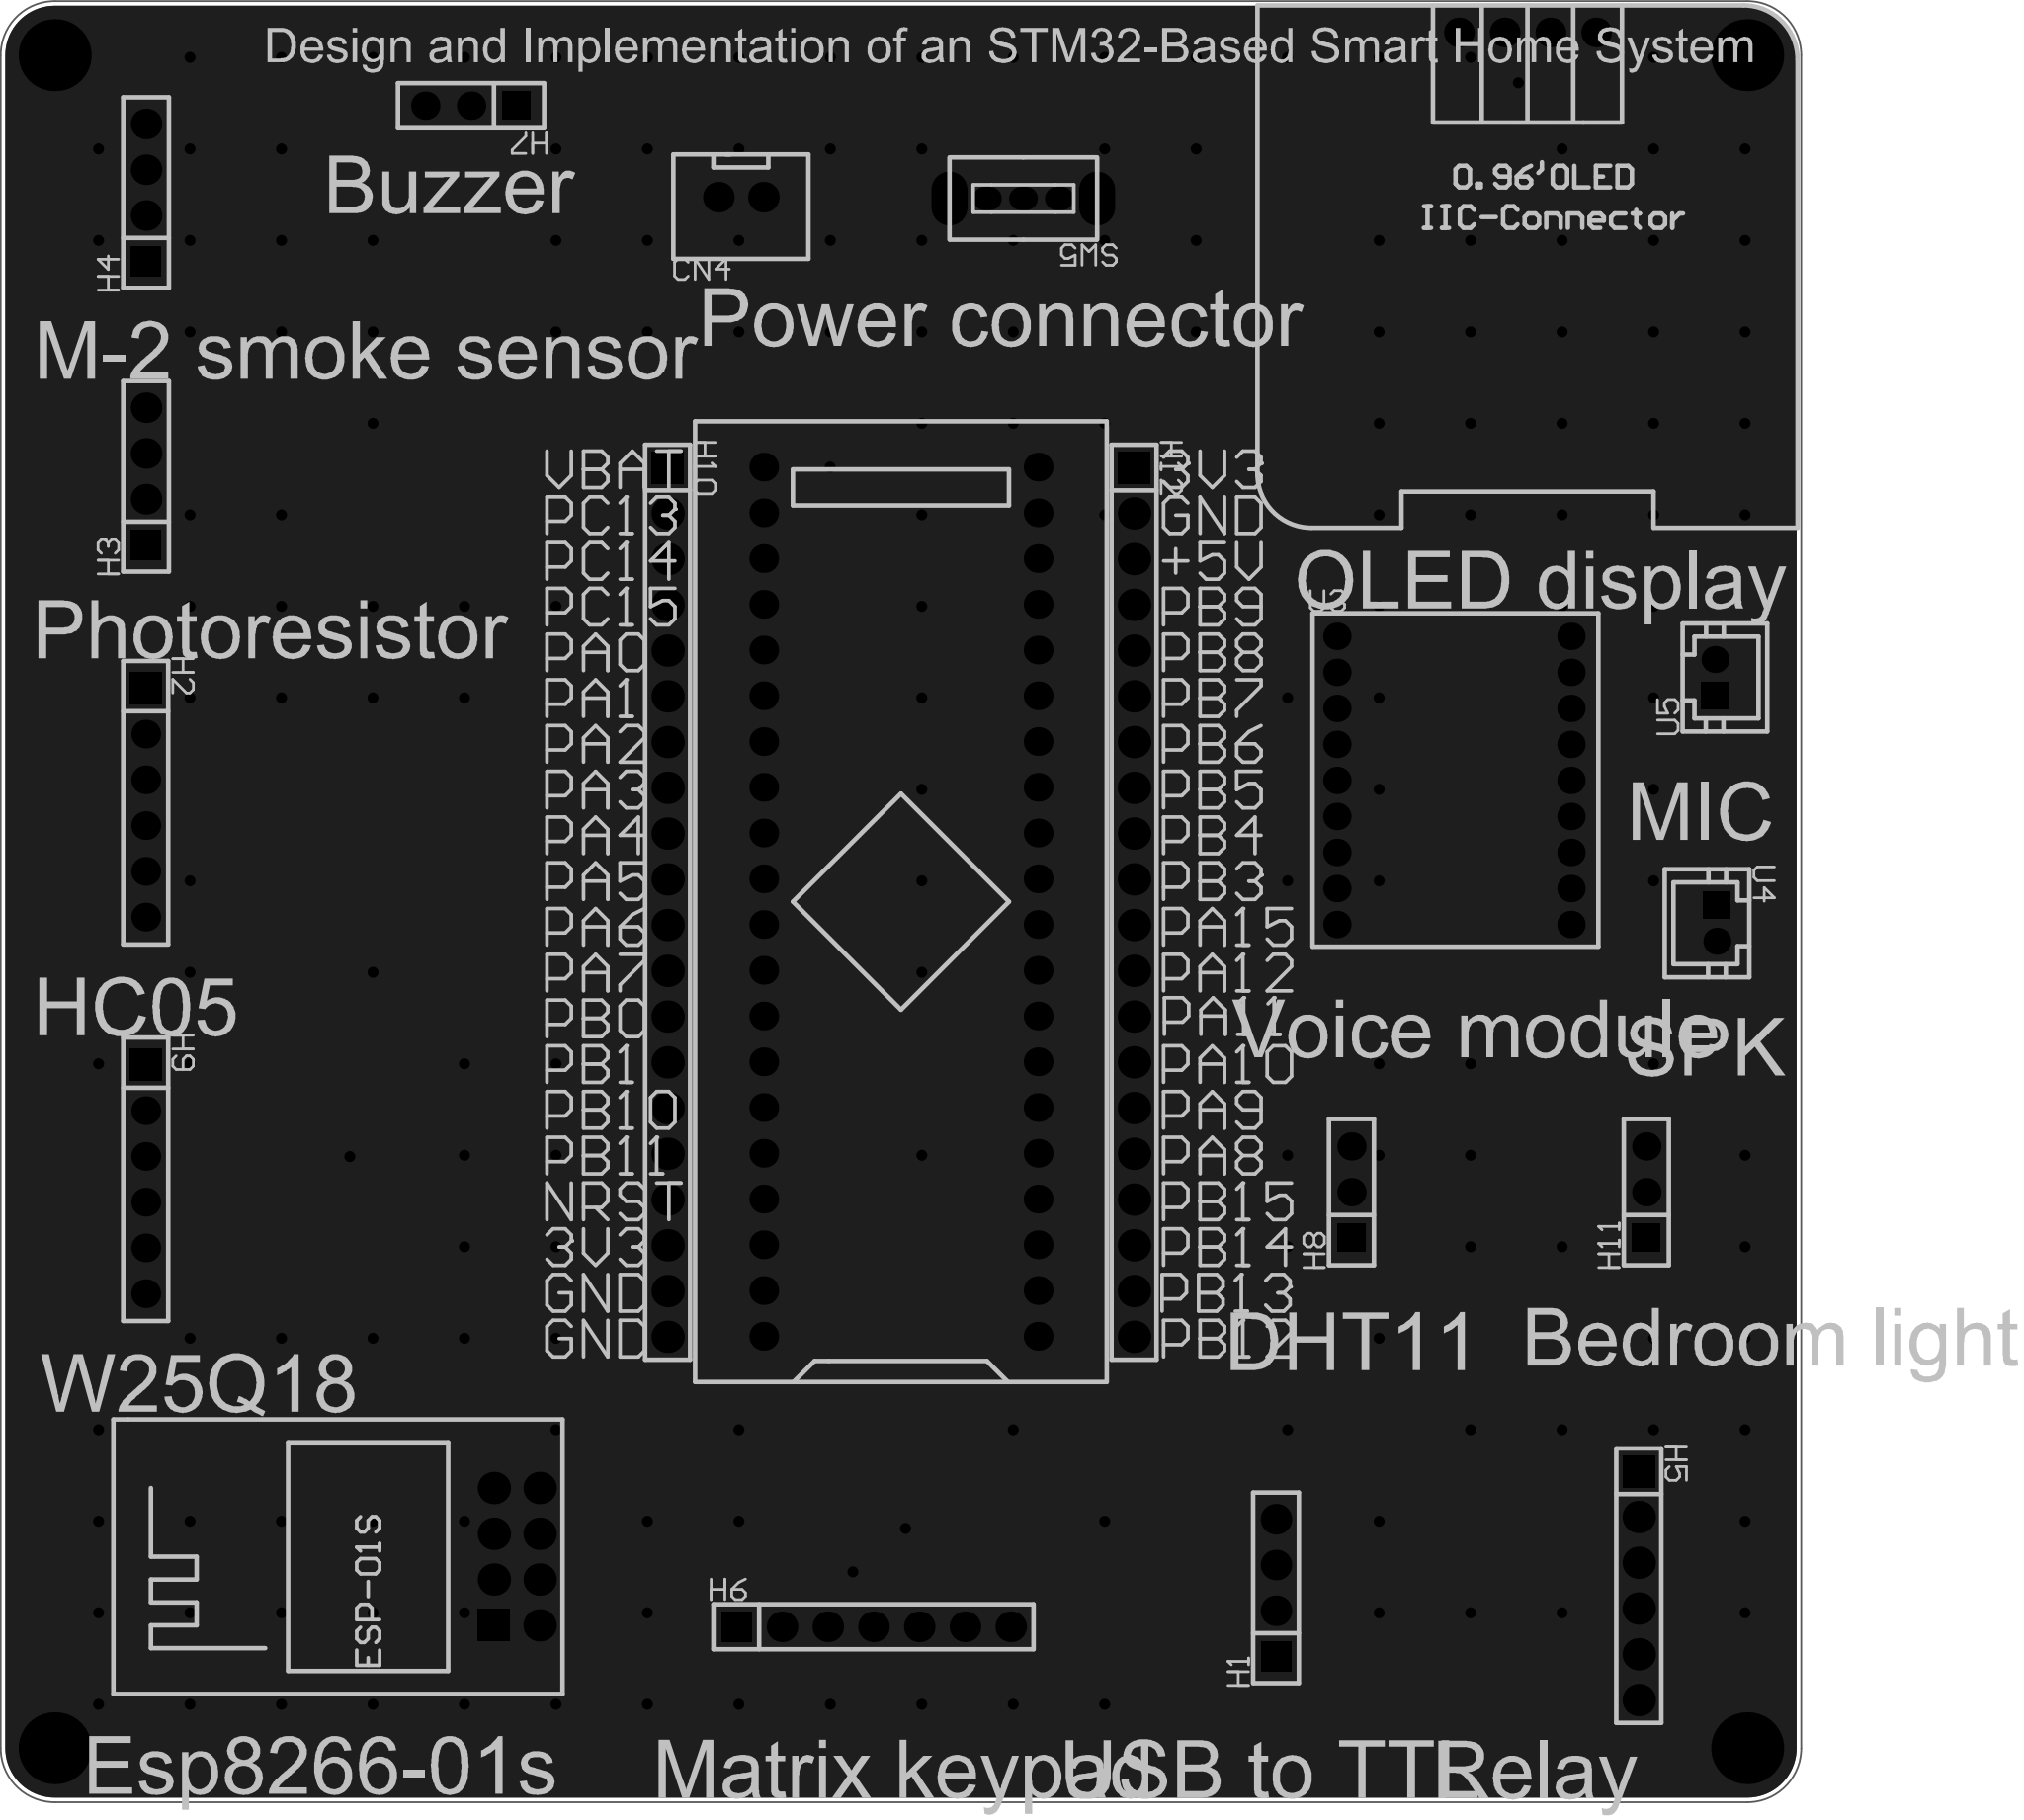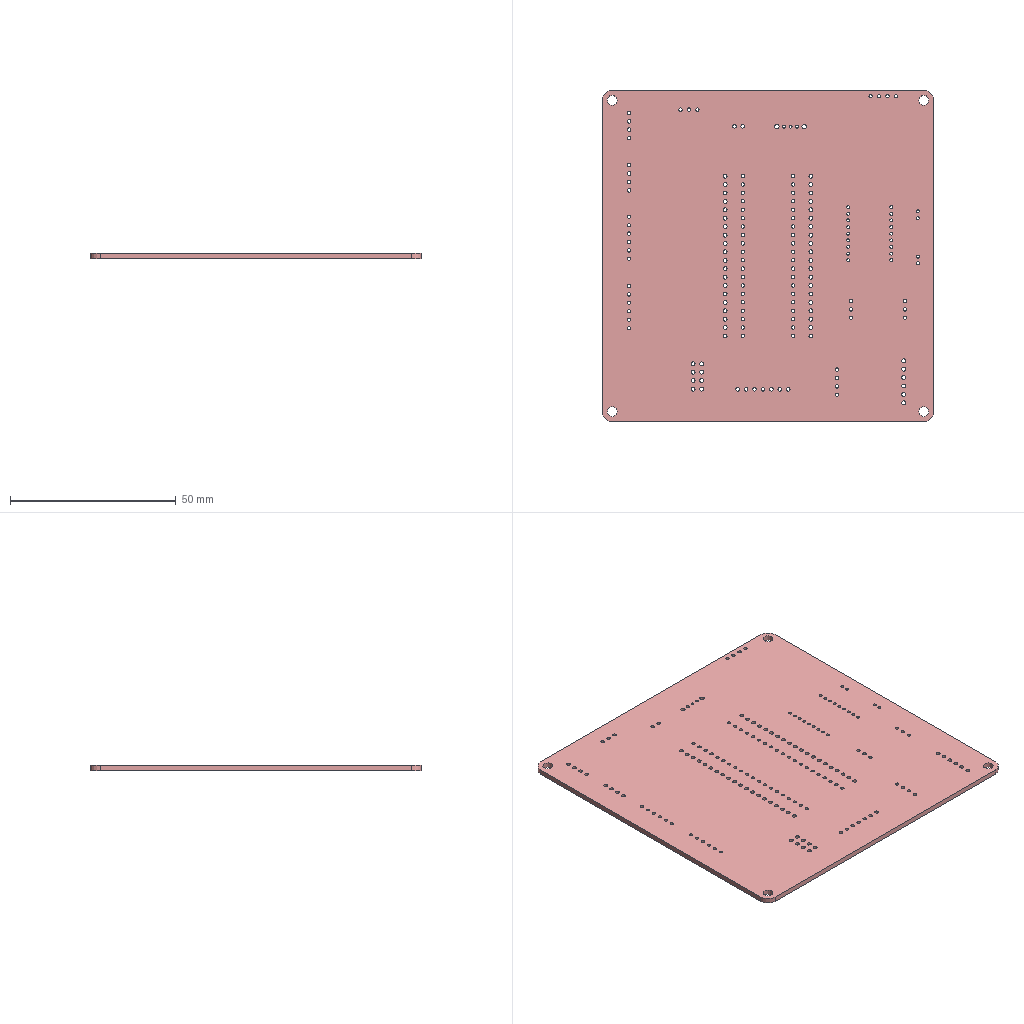Circuit board layout | Altium Designer | box 100 x 100 x 1.6 mm
Layer stack:
# Altium Designer layer stack of  (unit mm; dielectric type: 0 none, 1 core, 2 prepreg, 3 surface material)
index,name,kind,layer,copper_thickness_mm,dielectric_type,dielectric_thickness_mm,dielectric_material,dielectric_constant
0,Top Paste Mask Layer,other,,,,,,
1,Top Silkscreen Layer,other,,,,,,
2,Top Solder Mask Layer,dielectric,,,3,0.01,,3.3
3,Top Layer,copper,Top Layer,0.035,,,,
4,Dielectric1,dielectric,,,3,1.51,FR4,4.5
5,Bottom Layer,copper,Bottom Layer,0.035,,,,
6,Bottom Solder Mask Layer,dielectric,,,3,0.01,,3.3
7,Bottom Silkscreen Layer,other,,,,,,
8,Bottom Paste Mask Layer,other,,,,,,
# drill layer pairs: low layer,high layer
drill_pair,Top Layer,Bottom Layer
Part placement:
Designator,Comment,Layer,Footprint,Center-X(mm),Center-Y(mm),Rotation
U1,STM32F103C8T6-Card,TopLayer,CONN-TH_L53.3-W22.9_STM32F103C8T6-CARD,141.351,130.937,90
U2,ESP-01S,TopLayer,WIFIM-TH_ESP-01S,120.015,94.57,90
OLED1,,TopLayer,0.96OLED_4P,176.149,179.197,0
H11,,TopLayer,HDR-TH_3P-P2.54-V-F,182.746,114.808,90
CN4,XH2.54*2P_THT,TopLayer,CONN-TH_2P-P2.50-XH2.54-2P,132.461,170.053,0
U3,CON2.0MM-PAD-18,TopLayer,CONN-TH_18P-P2.00_C9900078766,172.062,137.668,90
SW5,,TopLayer,拨动开关,148.148,169.978,180
H1,,TopLayer,HDR-TH_4P-P2.54-V-F,162.179,92.837,90
H2,,TopLayer,HDR-TH_6P-P2.54-V-F,99.406,136.431,270
H3,,TopLayer,HDR-TH_4P-P2.54-V-F,99.426,154.553,90
H4,,TopLayer,HDR-TH_4P-P2.54-V-F,99.426,170.307,90
H5,,TopLayer,HDR-TH_6P-P2.54-V-M-1,182.328,92.962,270
H6,,TopLayer,HDR-TH_7P-P2.54-V-M,139.827,90.678,0
H7,,TopLayer,HDR-TH_3P-P2.54-V-F,117.475,175.133,180
H8,,TopLayer,HDR-TH_3P-P2.54-V-F,166.37,114.808,90
H9,,TopLayer,HDR-TH_6P-P2.54-V-F,99.406,115.524,270
H10,,TopLayer,HDR-TH_20P-P2.54-V-M-1,128.394,130.907,270
H12,,TopLayer,HDR-TH_20P-P2.54-V-M-1,154.294,130.907,270
U4,PH2.0-2P,TopLayer,CONN-TH_2P-P2.00_BOSSIE_BX-PH2.0-2PZZ,186.666,129.738,270
U5,PH2.0-2P,TopLayer,CONN-TH_2P-P2.00_BOSSIE_BX-PH2.0-2PZZ,186.563,143.383,90
Pad and via stacks:
# Altium Designer via and pad stacks of  (unit mm). Each distinct definition once, with the count of objects using it.
# via: kind,start_layer,end_layer,hole_mm,diameter_mm,mode(0 simple;1 top-mid-bottom;2 full stack),diameter_per_layer,count,example_net
# pad: kind,layer,hole_mm,hole_type(0 round;1 square;2 slot),plating,top_size,top_shape(1 round;2 rect;3 octagon;9 rounded rect),mid_size,bottom_size,mode,footprint,size_per_layer,count,example
pad,Multi-Layer,3,0,plated,4x4,1,4x4,4x4,0,,,4,1
pad,Multi-Layer,1,0,plated,1.6x1.6,1,1.6x1.6,1.6x1.6,0,CONN-TH_L53.3-W22.9_STM32F103C8T6-CARD,,40,U1.1
pad,Multi-Layer,1.2,0,plated,1.8x1.8,2,1.8x1.8,1.8x1.8,0,WIFIM-TH_ESP-01S,,1,U2.1
pad,Multi-Layer,1.2,0,plated,1.8x1.8,1,1.8x1.8,1.8x1.8,0,WIFIM-TH_ESP-01S,,7,U2.2
pad,Multi-Layer,1,0,plated,1.65x1.65,1,1.65x1.65,1.65x1.65,0,0.96OLED_4P,,4,OLED1.4
pad,Multi-Layer,1.02,0,plated,1.575x1.575,1,1.575x1.575,1.575x1.575,0,HDR-TH_3P-P2.54-V-F,,6,H11.3
pad,Multi-Layer,1.02,0,plated,1.575x1.575,2,1.575x1.575,1.575x1.575,0,HDR-TH_3P-P2.54-V-F,,3,H11.1
pad,Multi-Layer,1.05,0,plated,1.7x1.7,1,1.7x1.7,1.7x1.7,0,CONN-TH_2P-P2.50-XH2.54-2P,,2,CN4.2
pad,Multi-Layer,0.9,0,plated,1.524x1.524,1,1.524x1.524,1.524x1.524,0,CONN-TH_18P-P2.00_C9900078766,,18,U3.1
pad,Multi-Layer,0.8992,0,plated,1.6x1.3,1,1.6x1.3,1.6x1.3,0,\u00B2\u00A6\u00B6\u00AF\u00BF\u00AA\u00B9\u00D8,,3,SW5.1
pad,Multi-Layer,1.3,0,plated,3x1.999,1,3x1.999,3x1.999,0,\u00B2\u00A6\u00B6\u00AF\u00BF\u00AA\u00B9\u00D8,,2,SW5.4
pad,Multi-Layer,1.1,0,plated,1.7x1.7,2,1.7x1.7,1.7x1.7,0,HDR-TH_4P-P2.54-V-F,,3,H1.1
pad,Multi-Layer,1.1,0,plated,1.7x1.7,1,1.7x1.7,1.7x1.7,0,HDR-TH_4P-P2.54-V-F,,9,H1.2
pad,Multi-Layer,1.02,0,plated,1.6x1.6,1,1.6x1.6,1.6x1.6,0,HDR-TH_6P-P2.54-V-F,,10,H2.6
pad,Multi-Layer,1.02,0,plated,1.8x1.8,2,1.8x1.8,1.8x1.8,0,HDR-TH_6P-P2.54-V-F,,2,H2.1
pad,Multi-Layer,1.2,0,plated,1.8x1.8,1,1.8x1.8,1.8x1.8,0,HDR-TH_6P-P2.54-V-M-1,,5,H5.6
pad,Multi-Layer,1.2,0,plated,1.8x1.8,2,1.8x1.8,1.8x1.8,0,HDR-TH_6P-P2.54-V-M-1,,1,H5.1
pad,Multi-Layer,1.1,0,plated,1.7x1.7,2,1.7x1.7,1.7x1.7,0,HDR-TH_7P-P2.54-V-M,,1,H6.1
pad,Multi-Layer,1.1,0,plated,1.7x1.7,1,1.7x1.7,1.7x1.7,0,HDR-TH_7P-P2.54-V-M,,6,H6.2
pad,Multi-Layer,1.2,0,plated,1.8x1.8,1,1.8x1.8,1.8x1.8,0,HDR-TH_20P-P2.54-V-M-1,,38,H10.20
pad,Multi-Layer,1.2,0,plated,1.8x1.8,2,1.8x1.8,1.8x1.8,0,HDR-TH_20P-P2.54-V-M-1,,2,H10.1
pad,Multi-Layer,0.9,0,plated,1.5x1.5,2,1.5x1.5,1.5x1.5,0,CONN-TH_2P-P2.00_BOSSIE_BX-PH2.0-2PZZ,,2,U4.1
pad,Multi-Layer,0.9,0,plated,1.5x1.5,1,1.5x1.5,1.5x1.5,0,CONN-TH_2P-P2.00_BOSSIE_BX-PH2.0-2PZZ,,2,U4.2
via,Top Layer,Bottom Layer,0.3048,0.61,0,,181,PB9
Copper pours:
name,layer,net,type(0 solid;1 hatched;2 none)
Bottom Layer-GND,Bottom Layer,GND,0
Top Layer-GND,Top Layer,GND,0